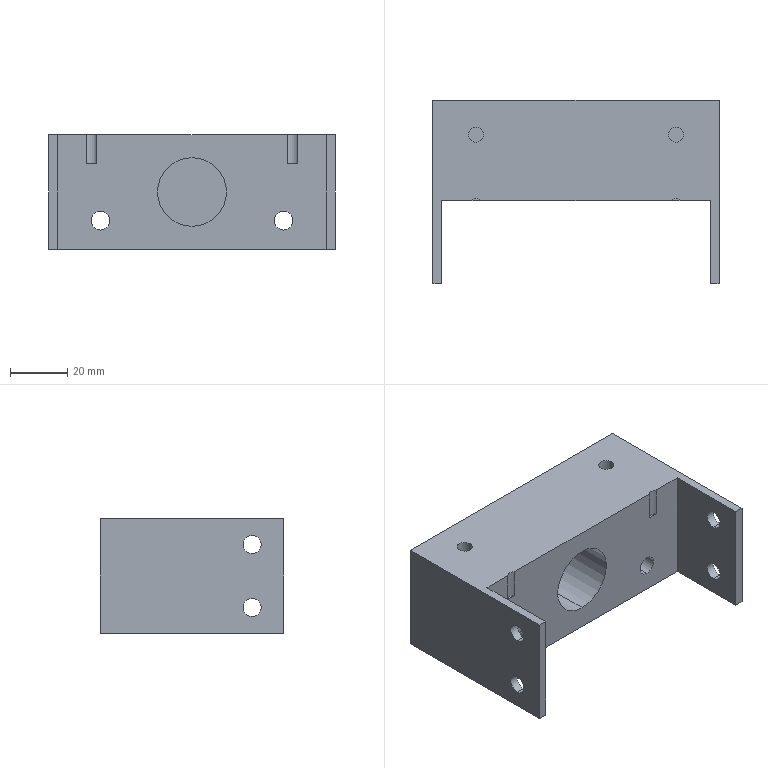Part | SolidWorks | features BaseBody 1 | 1 solid | 47 faces | box 100 x 64 x 40 mm | volume 128362 mm3 | cylinder 28 | plane 19 | commonest cylinder face diameters 4.3 x8 6.3 x8 5.3 x6 6.6 x4 24 x2
STEP:
#1=CARTESIAN_POINT('',(40.,24.8,9.85));
#2=VERTEX_POINT('',#1);
#3=CARTESIAN_POINT('',(40.,24.8,14.15));
#4=VERTEX_POINT('',#3);
#5=CARTESIAN_POINT('',(40.,24.8,12.));
#6=DIRECTION('',(0.,1.,0.));
#7=DIRECTION('',(0.,0.,1.));
#8=AXIS2_PLACEMENT_3D('',#5,#6,#7);
#9=CIRCLE('',#8,2.15);
#10=EDGE_CURVE('',#2,#4,#9,.T.);
#11=ORIENTED_EDGE('',*,*,#10,.F.);
#12=CARTESIAN_POINT('',(40.,32.,9.85));
#13=VERTEX_POINT('',#12);
#14=CARTESIAN_POINT('',(40.,24.8,9.85));
#15=DIRECTION('',(0.,1.,0.));
#16=VECTOR('',#15,1000.);
#17=LINE('',#14,#16);
#18=EDGE_CURVE('',#2,#13,#17,.T.);
#19=ORIENTED_EDGE('',*,*,#18,.T.);
#20=CARTESIAN_POINT('',(40.,32.,14.15));
#21=VERTEX_POINT('',#20);
#22=CARTESIAN_POINT('',(40.,32.,12.));
#23=DIRECTION('',(0.,-1.,0.));
#24=DIRECTION('',(0.,0.,1.));
#25=AXIS2_PLACEMENT_3D('',#22,#23,#24);
#26=CIRCLE('',#25,2.15);
#27=EDGE_CURVE('',#21,#13,#26,.T.);
#28=ORIENTED_EDGE('',*,*,#27,.F.);
#29=CARTESIAN_POINT('',(40.,24.8,14.15));
#30=DIRECTION('',(0.,1.,0.));
#31=VECTOR('',#30,1000.);
#32=LINE('',#29,#31);
#33=EDGE_CURVE('',#4,#21,#32,.T.);
#34=ORIENTED_EDGE('',*,*,#33,.F.);
#35=EDGE_LOOP('',(#11,#19,#28,#34));
#36=FACE_OUTER_BOUND('',#35,.T.);
#37=CARTESIAN_POINT('',(40.,24.8,12.));
#38=DIRECTION('',(0.,1.,0.));
#39=DIRECTION('',(0.,0.,1.));
#40=AXIS2_PLACEMENT_3D('',#37,#38,#39);
#41=CYLINDRICAL_SURFACE('',#40,2.15);
#42=ADVANCED_FACE('',(#36),#41,.F.);
#43=CARTESIAN_POINT('',(32.,-3.,-13.3));
#44=VERTEX_POINT('',#43);
#45=CARTESIAN_POINT('',(32.,-3.,-6.7));
#46=VERTEX_POINT('',#45);
#47=CARTESIAN_POINT('',(32.,-3.,-10.));
#48=DIRECTION('',(0.,1.,0.));
#49=DIRECTION('',(0.,0.,1.));
#50=AXIS2_PLACEMENT_3D('',#47,#48,#49);
#51=CIRCLE('',#50,3.3);
#52=EDGE_CURVE('',#44,#46,#51,.T.);
#53=ORIENTED_EDGE('',*,*,#52,.F.);
#54=CARTESIAN_POINT('',(32.,32.,-13.3));
#55=VERTEX_POINT('',#54);
#56=CARTESIAN_POINT('',(32.,-33.,-13.3));
#57=DIRECTION('',(0.,1.,0.));
#58=VECTOR('',#57,1000.);
#59=LINE('',#56,#58);
#60=EDGE_CURVE('',#44,#55,#59,.T.);
#61=ORIENTED_EDGE('',*,*,#60,.T.);
#62=CARTESIAN_POINT('',(32.,32.,-6.7));
#63=VERTEX_POINT('',#62);
#64=CARTESIAN_POINT('',(32.,32.,-10.));
#65=DIRECTION('',(0.,-1.,0.));
#66=DIRECTION('',(0.,0.,1.));
#67=AXIS2_PLACEMENT_3D('',#64,#65,#66);
#68=CIRCLE('',#67,3.3);
#69=EDGE_CURVE('',#63,#55,#68,.T.);
#70=ORIENTED_EDGE('',*,*,#69,.F.);
#71=CARTESIAN_POINT('',(32.,-33.,-6.7));
#72=DIRECTION('',(0.,1.,0.));
#73=VECTOR('',#72,1000.);
#74=LINE('',#71,#73);
#75=EDGE_CURVE('',#46,#63,#74,.T.);
#76=ORIENTED_EDGE('',*,*,#75,.F.);
#77=EDGE_LOOP('',(#53,#61,#70,#76));
#78=FACE_OUTER_BOUND('',#77,.T.);
#79=CARTESIAN_POINT('',(32.,-33.,-10.));
#80=DIRECTION('',(0.,1.,0.));
#81=DIRECTION('',(0.,0.,1.));
#82=AXIS2_PLACEMENT_3D('',#79,#80,#81);
#83=CYLINDRICAL_SURFACE('',#82,3.3);
#84=ADVANCED_FACE('',(#78),#83,.F.);
#85=CARTESIAN_POINT('',(40.,24.8,-14.15));
#86=VERTEX_POINT('',#85);
#87=CARTESIAN_POINT('',(40.,24.8,-9.85));
#88=VERTEX_POINT('',#87);
#89=CARTESIAN_POINT('',(40.,24.8,-12.));
#90=DIRECTION('',(0.,1.,0.));
#91=DIRECTION('',(0.,0.,1.));
#92=AXIS2_PLACEMENT_3D('',#89,#90,#91);
#93=CIRCLE('',#92,2.15);
#94=EDGE_CURVE('',#86,#88,#93,.T.);
#95=ORIENTED_EDGE('',*,*,#94,.F.);
#96=CARTESIAN_POINT('',(40.,32.,-14.15));
#97=VERTEX_POINT('',#96);
#98=CARTESIAN_POINT('',(40.,24.8,-14.15));
#99=DIRECTION('',(0.,1.,0.));
#100=VECTOR('',#99,1000.);
#101=LINE('',#98,#100);
#102=EDGE_CURVE('',#86,#97,#101,.T.);
#103=ORIENTED_EDGE('',*,*,#102,.T.);
#104=CARTESIAN_POINT('',(40.,32.,-9.85));
#105=VERTEX_POINT('',#104);
#106=CARTESIAN_POINT('',(40.,32.,-12.));
#107=DIRECTION('',(0.,-1.,0.));
#108=DIRECTION('',(0.,0.,1.));
#109=AXIS2_PLACEMENT_3D('',#106,#107,#108);
#110=CIRCLE('',#109,2.15);
#111=EDGE_CURVE('',#105,#97,#110,.T.);
#112=ORIENTED_EDGE('',*,*,#111,.F.);
#113=CARTESIAN_POINT('',(40.,24.8,-9.85));
#114=DIRECTION('',(0.,1.,0.));
#115=VECTOR('',#114,1000.);
#116=LINE('',#113,#115);
#117=EDGE_CURVE('',#88,#105,#116,.T.);
#118=ORIENTED_EDGE('',*,*,#117,.F.);
#119=EDGE_LOOP('',(#95,#103,#112,#118));
#120=FACE_OUTER_BOUND('',#119,.T.);
#121=CARTESIAN_POINT('',(40.,24.8,-12.));
#122=DIRECTION('',(0.,1.,0.));
#123=DIRECTION('',(0.,0.,1.));
#124=AXIS2_PLACEMENT_3D('',#121,#122,#123);
#125=CYLINDRICAL_SURFACE('',#124,2.15);
#126=ADVANCED_FACE('',(#120),#125,.F.);
#127=CARTESIAN_POINT('',(-40.,24.8,9.85));
#128=VERTEX_POINT('',#127);
#129=CARTESIAN_POINT('',(-40.,24.8,14.15));
#130=VERTEX_POINT('',#129);
#131=CARTESIAN_POINT('',(-40.,24.8,12.));
#132=DIRECTION('',(0.,1.,0.));
#133=DIRECTION('',(0.,0.,1.));
#134=AXIS2_PLACEMENT_3D('',#131,#132,#133);
#135=CIRCLE('',#134,2.15);
#136=EDGE_CURVE('',#128,#130,#135,.T.);
#137=ORIENTED_EDGE('',*,*,#136,.F.);
#138=CARTESIAN_POINT('',(-40.,32.,9.85));
#139=VERTEX_POINT('',#138);
#140=CARTESIAN_POINT('',(-40.,24.8,9.85));
#141=DIRECTION('',(0.,1.,0.));
#142=VECTOR('',#141,1000.);
#143=LINE('',#140,#142);
#144=EDGE_CURVE('',#128,#139,#143,.T.);
#145=ORIENTED_EDGE('',*,*,#144,.T.);
#146=CARTESIAN_POINT('',(-40.,32.,14.15));
#147=VERTEX_POINT('',#146);
#148=CARTESIAN_POINT('',(-40.,32.,12.));
#149=DIRECTION('',(0.,-1.,0.));
#150=DIRECTION('',(0.,0.,1.));
#151=AXIS2_PLACEMENT_3D('',#148,#149,#150);
#152=CIRCLE('',#151,2.15);
#153=EDGE_CURVE('',#147,#139,#152,.T.);
#154=ORIENTED_EDGE('',*,*,#153,.F.);
#155=CARTESIAN_POINT('',(-40.,24.8,14.15));
#156=DIRECTION('',(0.,1.,0.));
#157=VECTOR('',#156,1000.);
#158=LINE('',#155,#157);
#159=EDGE_CURVE('',#130,#147,#158,.T.);
#160=ORIENTED_EDGE('',*,*,#159,.F.);
#161=EDGE_LOOP('',(#137,#145,#154,#160));
#162=FACE_OUTER_BOUND('',#161,.T.);
#163=CARTESIAN_POINT('',(-40.,24.8,12.));
#164=DIRECTION('',(0.,1.,0.));
#165=DIRECTION('',(0.,0.,1.));
#166=AXIS2_PLACEMENT_3D('',#163,#164,#165);
#167=CYLINDRICAL_SURFACE('',#166,2.15);
#168=ADVANCED_FACE('',(#162),#167,.F.);
#169=CARTESIAN_POINT('',(-32.,-3.,-13.3));
#170=VERTEX_POINT('',#169);
#171=CARTESIAN_POINT('',(-32.,-3.,-6.7));
#172=VERTEX_POINT('',#171);
#173=CARTESIAN_POINT('',(-32.,-3.,-10.));
#174=DIRECTION('',(0.,1.,0.));
#175=DIRECTION('',(0.,0.,1.));
#176=AXIS2_PLACEMENT_3D('',#173,#174,#175);
#177=CIRCLE('',#176,3.3);
#178=EDGE_CURVE('',#170,#172,#177,.T.);
#179=ORIENTED_EDGE('',*,*,#178,.F.);
#180=CARTESIAN_POINT('',(-32.,32.,-13.3));
#181=VERTEX_POINT('',#180);
#182=CARTESIAN_POINT('',(-32.,-33.,-13.3));
#183=DIRECTION('',(0.,1.,0.));
#184=VECTOR('',#183,1000.);
#185=LINE('',#182,#184);
#186=EDGE_CURVE('',#170,#181,#185,.T.);
#187=ORIENTED_EDGE('',*,*,#186,.T.);
#188=CARTESIAN_POINT('',(-32.,32.,-6.7));
#189=VERTEX_POINT('',#188);
#190=CARTESIAN_POINT('',(-32.,32.,-10.));
#191=DIRECTION('',(0.,-1.,0.));
#192=DIRECTION('',(0.,0.,1.));
#193=AXIS2_PLACEMENT_3D('',#190,#191,#192);
#194=CIRCLE('',#193,3.3);
#195=EDGE_CURVE('',#189,#181,#194,.T.);
#196=ORIENTED_EDGE('',*,*,#195,.F.);
#197=CARTESIAN_POINT('',(-32.,-33.,-6.7));
#198=DIRECTION('',(0.,1.,0.));
#199=VECTOR('',#198,1000.);
#200=LINE('',#197,#199);
#201=EDGE_CURVE('',#172,#189,#200,.T.);
#202=ORIENTED_EDGE('',*,*,#201,.F.);
#203=EDGE_LOOP('',(#179,#187,#196,#202));
#204=FACE_OUTER_BOUND('',#203,.T.);
#205=CARTESIAN_POINT('',(-32.,-33.,-10.));
#206=DIRECTION('',(0.,1.,0.));
#207=DIRECTION('',(0.,0.,1.));
#208=AXIS2_PLACEMENT_3D('',#205,#206,#207);
#209=CYLINDRICAL_SURFACE('',#208,3.3);
#210=ADVANCED_FACE('',(#204),#209,.F.);
#211=CARTESIAN_POINT('',(-40.,24.8,-14.15));
#212=VERTEX_POINT('',#211);
#213=CARTESIAN_POINT('',(-40.,24.8,-9.85));
#214=VERTEX_POINT('',#213);
#215=CARTESIAN_POINT('',(-40.,24.8,-12.));
#216=DIRECTION('',(0.,1.,0.));
#217=DIRECTION('',(0.,0.,1.));
#218=AXIS2_PLACEMENT_3D('',#215,#216,#217);
#219=CIRCLE('',#218,2.15);
#220=EDGE_CURVE('',#212,#214,#219,.T.);
#221=ORIENTED_EDGE('',*,*,#220,.F.);
#222=CARTESIAN_POINT('',(-40.,32.,-14.15));
#223=VERTEX_POINT('',#222);
#224=CARTESIAN_POINT('',(-40.,24.8,-14.15));
#225=DIRECTION('',(0.,1.,0.));
#226=VECTOR('',#225,1000.);
#227=LINE('',#224,#226);
#228=EDGE_CURVE('',#212,#223,#227,.T.);
#229=ORIENTED_EDGE('',*,*,#228,.T.);
#230=CARTESIAN_POINT('',(-40.,32.,-9.85));
#231=VERTEX_POINT('',#230);
#232=CARTESIAN_POINT('',(-40.,32.,-12.));
#233=DIRECTION('',(0.,-1.,0.));
#234=DIRECTION('',(0.,0.,1.));
#235=AXIS2_PLACEMENT_3D('',#232,#233,#234);
#236=CIRCLE('',#235,2.15);
#237=EDGE_CURVE('',#231,#223,#236,.T.);
#238=ORIENTED_EDGE('',*,*,#237,.F.);
#239=CARTESIAN_POINT('',(-40.,24.8,-9.85));
#240=DIRECTION('',(0.,1.,0.));
#241=VECTOR('',#240,1000.);
#242=LINE('',#239,#241);
#243=EDGE_CURVE('',#214,#231,#242,.T.);
#244=ORIENTED_EDGE('',*,*,#243,.F.);
#245=EDGE_LOOP('',(#221,#229,#238,#244));
#246=FACE_OUTER_BOUND('',#245,.T.);
#247=CARTESIAN_POINT('',(-40.,24.8,-12.));
#248=DIRECTION('',(0.,1.,0.));
#249=DIRECTION('',(0.,0.,1.));
#250=AXIS2_PLACEMENT_3D('',#247,#248,#249);
#251=CYLINDRICAL_SURFACE('',#250,2.15);
#252=ADVANCED_FACE('',(#246),#251,.F.);
#253=CARTESIAN_POINT('',(47.,-21.,14.15));
#254=VERTEX_POINT('',#253);
#255=CARTESIAN_POINT('',(47.,-21.,7.85));
#256=VERTEX_POINT('',#255);
#257=CARTESIAN_POINT('',(47.,-21.,11.));
#258=DIRECTION('',(1.,0.,0.));
#259=DIRECTION('',(0.,0.,-1.));
#260=AXIS2_PLACEMENT_3D('',#257,#258,#259);
#261=CIRCLE('',#260,3.15);
#262=EDGE_CURVE('',#254,#256,#261,.T.);
#263=ORIENTED_EDGE('',*,*,#262,.F.);
#264=CARTESIAN_POINT('',(50.,-21.,14.15));
#265=VERTEX_POINT('',#264);
#266=CARTESIAN_POINT('',(-51.,-21.,14.15));
#267=DIRECTION('',(1.,0.,0.));
#268=VECTOR('',#267,1000.);
#269=LINE('',#266,#268);
#270=EDGE_CURVE('',#254,#265,#269,.T.);
#271=ORIENTED_EDGE('',*,*,#270,.T.);
#272=CARTESIAN_POINT('',(50.,-21.,7.85));
#273=VERTEX_POINT('',#272);
#274=CARTESIAN_POINT('',(50.,-21.,11.));
#275=DIRECTION('',(-1.,0.,0.));
#276=DIRECTION('',(0.,0.,-1.));
#277=AXIS2_PLACEMENT_3D('',#274,#275,#276);
#278=CIRCLE('',#277,3.15);
#279=EDGE_CURVE('',#273,#265,#278,.T.);
#280=ORIENTED_EDGE('',*,*,#279,.F.);
#281=CARTESIAN_POINT('',(-51.,-21.,7.85));
#282=DIRECTION('',(1.,0.,0.));
#283=VECTOR('',#282,1000.);
#284=LINE('',#281,#283);
#285=EDGE_CURVE('',#256,#273,#284,.T.);
#286=ORIENTED_EDGE('',*,*,#285,.F.);
#287=EDGE_LOOP('',(#263,#271,#280,#286));
#288=FACE_OUTER_BOUND('',#287,.T.);
#289=CARTESIAN_POINT('',(-51.,-21.,11.));
#290=DIRECTION('',(1.,0.,0.));
#291=DIRECTION('',(0.,0.,-1.));
#292=AXIS2_PLACEMENT_3D('',#289,#290,#291);
#293=CYLINDRICAL_SURFACE('',#292,3.15);
#294=ADVANCED_FACE('',(#288),#293,.F.);
#295=CARTESIAN_POINT('',(47.,-21.,-7.85));
#296=VERTEX_POINT('',#295);
#297=CARTESIAN_POINT('',(47.,-21.,-14.15));
#298=VERTEX_POINT('',#297);
#299=CARTESIAN_POINT('',(47.,-21.,-11.));
#300=DIRECTION('',(1.,0.,0.));
#301=DIRECTION('',(0.,0.,-1.));
#302=AXIS2_PLACEMENT_3D('',#299,#300,#301);
#303=CIRCLE('',#302,3.15);
#304=EDGE_CURVE('',#296,#298,#303,.T.);
#305=ORIENTED_EDGE('',*,*,#304,.F.);
#306=CARTESIAN_POINT('',(50.,-21.,-7.85));
#307=VERTEX_POINT('',#306);
#308=CARTESIAN_POINT('',(-51.,-21.,-7.85));
#309=DIRECTION('',(1.,0.,0.));
#310=VECTOR('',#309,1000.);
#311=LINE('',#308,#310);
#312=EDGE_CURVE('',#296,#307,#311,.T.);
#313=ORIENTED_EDGE('',*,*,#312,.T.);
#314=CARTESIAN_POINT('',(50.,-21.,-14.15));
#315=VERTEX_POINT('',#314);
#316=CARTESIAN_POINT('',(50.,-21.,-11.));
#317=DIRECTION('',(-1.,0.,0.));
#318=DIRECTION('',(0.,0.,-1.));
#319=AXIS2_PLACEMENT_3D('',#316,#317,#318);
#320=CIRCLE('',#319,3.15);
#321=EDGE_CURVE('',#315,#307,#320,.T.);
#322=ORIENTED_EDGE('',*,*,#321,.F.);
#323=CARTESIAN_POINT('',(-51.,-21.,-14.15));
#324=DIRECTION('',(1.,0.,0.));
#325=VECTOR('',#324,1000.);
#326=LINE('',#323,#325);
#327=EDGE_CURVE('',#298,#315,#326,.T.);
#328=ORIENTED_EDGE('',*,*,#327,.F.);
#329=EDGE_LOOP('',(#305,#313,#322,#328));
#330=FACE_OUTER_BOUND('',#329,.T.);
#331=CARTESIAN_POINT('',(-51.,-21.,-11.));
#332=DIRECTION('',(1.,0.,0.));
#333=DIRECTION('',(0.,0.,-1.));
#334=AXIS2_PLACEMENT_3D('',#331,#332,#333);
#335=CYLINDRICAL_SURFACE('',#334,3.15);
#336=ADVANCED_FACE('',(#330),#335,.F.);
#337=CARTESIAN_POINT('',(32.35,20.,9.8));
#338=VERTEX_POINT('',#337);
#339=CARTESIAN_POINT('',(37.65,20.,9.8));
#340=VERTEX_POINT('',#339);
#341=CARTESIAN_POINT('',(35.,20.,9.8));
#342=DIRECTION('',(0.,0.,1.));
#343=DIRECTION('',(1.,0.,0.));
#344=AXIS2_PLACEMENT_3D('',#341,#342,#343);
#345=CIRCLE('',#344,2.65);
#346=EDGE_CURVE('',#338,#340,#345,.T.);
#347=ORIENTED_EDGE('',*,*,#346,.F.);
#348=CARTESIAN_POINT('',(32.35,20.,20.));
#349=VERTEX_POINT('',#348);
#350=CARTESIAN_POINT('',(32.35,20.,9.8));
#351=DIRECTION('',(0.,0.,1.));
#352=VECTOR('',#351,1000.);
#353=LINE('',#350,#352);
#354=EDGE_CURVE('',#338,#349,#353,.T.);
#355=ORIENTED_EDGE('',*,*,#354,.T.);
#356=CARTESIAN_POINT('',(37.65,20.,20.));
#357=VERTEX_POINT('',#356);
#358=CARTESIAN_POINT('',(35.,20.,20.));
#359=DIRECTION('',(0.,0.,-1.));
#360=DIRECTION('',(1.,0.,0.));
#361=AXIS2_PLACEMENT_3D('',#358,#359,#360);
#362=CIRCLE('',#361,2.65);
#363=EDGE_CURVE('',#357,#349,#362,.T.);
#364=ORIENTED_EDGE('',*,*,#363,.F.);
#365=CARTESIAN_POINT('',(37.65,20.,9.8));
#366=DIRECTION('',(0.,0.,1.));
#367=VECTOR('',#366,1000.);
#368=LINE('',#365,#367);
#369=EDGE_CURVE('',#340,#357,#368,.T.);
#370=ORIENTED_EDGE('',*,*,#369,.F.);
#371=EDGE_LOOP('',(#347,#355,#364,#370));
#372=FACE_OUTER_BOUND('',#371,.T.);
#373=CARTESIAN_POINT('',(35.,20.,9.8));
#374=DIRECTION('',(0.,0.,1.));
#375=DIRECTION('',(1.,0.,0.));
#376=AXIS2_PLACEMENT_3D('',#373,#374,#375);
#377=CYLINDRICAL_SURFACE('',#376,2.65);
#378=ADVANCED_FACE('',(#372),#377,.F.);
#379=CARTESIAN_POINT('',(-37.65,20.,9.8));
#380=VERTEX_POINT('',#379);
#381=CARTESIAN_POINT('',(-32.35,20.,9.8));
#382=VERTEX_POINT('',#381);
#383=CARTESIAN_POINT('',(-35.,20.,9.8));
#384=DIRECTION('',(0.,0.,1.));
#385=DIRECTION('',(1.,0.,0.));
#386=AXIS2_PLACEMENT_3D('',#383,#384,#385);
#387=CIRCLE('',#386,2.65);
#388=EDGE_CURVE('',#380,#382,#387,.T.);
#389=ORIENTED_EDGE('',*,*,#388,.F.);
#390=CARTESIAN_POINT('',(-37.65,20.,20.));
#391=VERTEX_POINT('',#390);
#392=CARTESIAN_POINT('',(-37.65,20.,9.8));
#393=DIRECTION('',(0.,0.,1.));
#394=VECTOR('',#393,1000.);
#395=LINE('',#392,#394);
#396=EDGE_CURVE('',#380,#391,#395,.T.);
#397=ORIENTED_EDGE('',*,*,#396,.T.);
#398=CARTESIAN_POINT('',(-32.35,20.,20.));
#399=VERTEX_POINT('',#398);
#400=CARTESIAN_POINT('',(-35.,20.,20.));
#401=DIRECTION('',(0.,0.,-1.));
#402=DIRECTION('',(1.,0.,0.));
#403=AXIS2_PLACEMENT_3D('',#400,#401,#402);
#404=CIRCLE('',#403,2.65);
#405=EDGE_CURVE('',#399,#391,#404,.T.);
#406=ORIENTED_EDGE('',*,*,#405,.F.);
#407=CARTESIAN_POINT('',(-32.35,20.,9.8));
#408=DIRECTION('',(0.,0.,1.));
#409=VECTOR('',#408,1000.);
#410=LINE('',#407,#409);
#411=EDGE_CURVE('',#382,#399,#410,.T.);
#412=ORIENTED_EDGE('',*,*,#411,.F.);
#413=EDGE_LOOP('',(#389,#397,#406,#412));
#414=FACE_OUTER_BOUND('',#413,.T.);
#415=CARTESIAN_POINT('',(-35.,20.,9.8));
#416=DIRECTION('',(0.,0.,1.));
#417=DIRECTION('',(1.,0.,0.));
#418=AXIS2_PLACEMENT_3D('',#415,#416,#417);
#419=CYLINDRICAL_SURFACE('',#418,2.65);
#420=ADVANCED_FACE('',(#414),#419,.F.);
#421=CARTESIAN_POINT('',(-50.,-21.,7.85));
#422=VERTEX_POINT('',#421);
#423=CARTESIAN_POINT('',(-50.,-21.,14.15));
#424=VERTEX_POINT('',#423);
#425=CARTESIAN_POINT('',(-50.,-21.,11.));
#426=DIRECTION('',(-1.,0.,0.));
#427=DIRECTION('',(0.,0.,-1.));
#428=AXIS2_PLACEMENT_3D('',#425,#426,#427);
#429=CIRCLE('',#428,3.15);
#430=EDGE_CURVE('',#422,#424,#429,.T.);
#431=ORIENTED_EDGE('',*,*,#430,.T.);
#432=CARTESIAN_POINT('',(-47.,-21.,14.15));
#433=VERTEX_POINT('',#432);
#434=CARTESIAN_POINT('',(-51.,-21.,14.15));
#435=DIRECTION('',(1.,0.,0.));
#436=VECTOR('',#435,1000.);
#437=LINE('',#434,#436);
#438=EDGE_CURVE('',#424,#433,#437,.T.);
#439=ORIENTED_EDGE('',*,*,#438,.T.);
#440=CARTESIAN_POINT('',(-47.,-21.,7.85));
#441=VERTEX_POINT('',#440);
#442=CARTESIAN_POINT('',(-47.,-21.,11.));
#443=DIRECTION('',(-1.,0.,0.));
#444=DIRECTION('',(0.,0.,-1.));
#445=AXIS2_PLACEMENT_3D('',#442,#443,#444);
#446=CIRCLE('',#445,3.15);
#447=EDGE_CURVE('',#441,#433,#446,.T.);
#448=ORIENTED_EDGE('',*,*,#447,.F.);
#449=CARTESIAN_POINT('',(-51.,-21.,7.85));
#450=DIRECTION('',(1.,0.,0.));
#451=VECTOR('',#450,1000.);
#452=LINE('',#449,#451);
#453=EDGE_CURVE('',#422,#441,#452,.T.);
#454=ORIENTED_EDGE('',*,*,#453,.F.);
#455=EDGE_LOOP('',(#431,#439,#448,#454));
#456=FACE_OUTER_BOUND('',#455,.T.);
#457=CARTESIAN_POINT('',(-51.,-21.,11.));
#458=DIRECTION('',(1.,0.,0.));
#459=DIRECTION('',(0.,0.,-1.));
#460=AXIS2_PLACEMENT_3D('',#457,#458,#459);
#461=CYLINDRICAL_SURFACE('',#460,3.15);
#462=ADVANCED_FACE('',(#456),#461,.F.);
#463=CARTESIAN_POINT('',(-50.,-21.,-14.15));
#464=VERTEX_POINT('',#463);
#465=CARTESIAN_POINT('',(-50.,-21.,-7.85));
#466=VERTEX_POINT('',#465);
#467=CARTESIAN_POINT('',(-50.,-21.,-11.));
#468=DIRECTION('',(-1.,0.,0.));
#469=DIRECTION('',(0.,0.,-1.));
#470=AXIS2_PLACEMENT_3D('',#467,#468,#469);
#471=CIRCLE('',#470,3.15);
#472=EDGE_CURVE('',#464,#466,#471,.T.);
#473=ORIENTED_EDGE('',*,*,#472,.T.);
#474=CARTESIAN_POINT('',(-47.,-21.,-7.85));
#475=VERTEX_POINT('',#474);
#476=CARTESIAN_POINT('',(-51.,-21.,-7.85));
#477=DIRECTION('',(1.,0.,0.));
#478=VECTOR('',#477,1000.);
#479=LINE('',#476,#478);
#480=EDGE_CURVE('',#466,#475,#479,.T.);
#481=ORIENTED_EDGE('',*,*,#480,.T.);
#482=CARTESIAN_POINT('',(-47.,-21.,-14.15));
#483=VERTEX_POINT('',#482);
#484=CARTESIAN_POINT('',(-47.,-21.,-11.));
#485=DIRECTION('',(-1.,0.,0.));
#486=DIRECTION('',(0.,0.,-1.));
#487=AXIS2_PLACEMENT_3D('',#484,#485,#486);
#488=CIRCLE('',#487,3.15);
#489=EDGE_CURVE('',#483,#475,#488,.T.);
#490=ORIENTED_EDGE('',*,*,#489,.F.);
#491=CARTESIAN_POINT('',(-51.,-21.,-14.15));
#492=DIRECTION('',(1.,0.,0.));
#493=VECTOR('',#492,1000.);
#494=LINE('',#491,#493);
#495=EDGE_CURVE('',#464,#483,#494,.T.);
#496=ORIENTED_EDGE('',*,*,#495,.F.);
#497=EDGE_LOOP('',(#473,#481,#490,#496));
#498=FACE_OUTER_BOUND('',#497,.T.);
#499=CARTESIAN_POINT('',(-51.,-21.,-11.));
#500=DIRECTION('',(1.,0.,0.));
#501=DIRECTION('',(0.,0.,-1.));
#502=AXIS2_PLACEMENT_3D('',#499,#500,#501);
#503=CYLINDRICAL_SURFACE('',#502,3.15);
#504=ADVANCED_FACE('',(#498),#503,.F.);
#505=CARTESIAN_POINT('',(0.,-3.,12.));
#506=VERTEX_POINT('',#505);
#507=CARTESIAN_POINT('',(0.,-3.,-12.));
#508=VERTEX_POINT('',#507);
#509=CARTESIAN_POINT('',(0.,-3.,0.));
#510=DIRECTION('',(0.,-1.,0.));
#511=DIRECTION('',(0.,0.,1.));
#512=AXIS2_PLACEMENT_3D('',#509,#510,#511);
#513=CIRCLE('',#512,12.);
#514=EDGE_CURVE('',#506,#508,#513,.T.);
#515=ORIENTED_EDGE('',*,*,#514,.T.);
#516=CARTESIAN_POINT('',(0.,30.,-12.));
#517=VERTEX_POINT('',#516);
#518=CARTESIAN_POINT('',(0.,-14.,-12.));
#519=DIRECTION('',(0.,1.,0.));
#520=VECTOR('',#519,1000.);
#521=LINE('',#518,#520);
#522=EDGE_CURVE('',#508,#517,#521,.T.);
#523=ORIENTED_EDGE('',*,*,#522,.T.);
#524=CARTESIAN_POINT('',(0.,30.,12.));
#525=VERTEX_POINT('',#524);
#526=CARTESIAN_POINT('',(0.,30.,0.));
#527=DIRECTION('',(0.,-1.,0.));
#528=DIRECTION('',(0.,0.,1.));
#529=AXIS2_PLACEMENT_3D('',#526,#527,#528);
#530=CIRCLE('',#529,12.);
#531=EDGE_CURVE('',#525,#517,#530,.T.);
#532=ORIENTED_EDGE('',*,*,#531,.F.);
#533=CARTESIAN_POINT('',(0.,-14.,12.));
#534=DIRECTION('',(0.,1.,0.));
#535=VECTOR('',#534,1000.);
#536=LINE('',#533,#535);
#537=EDGE_CURVE('',#506,#525,#536,.T.);
#538=ORIENTED_EDGE('',*,*,#537,.F.);
#539=EDGE_LOOP('',(#515,#523,#532,#538));
#540=FACE_OUTER_BOUND('',#539,.T.);
#541=CARTESIAN_POINT('',(0.,-14.,0.));
#542=DIRECTION('',(0.,1.,0.));
#543=DIRECTION('',(0.,0.,1.));
#544=AXIS2_PLACEMENT_3D('',#541,#542,#543);
#545=CYLINDRICAL_SURFACE('',#544,12.);
#546=ADVANCED_FACE('',(#540),#545,.F.);
#547=ORIENTED_EDGE('',*,*,#27,.T.);
#548=CARTESIAN_POINT('',(40.,32.,12.));
#549=DIRECTION('',(0.,-1.,0.));
#550=DIRECTION('',(0.,0.,1.));
#551=AXIS2_PLACEMENT_3D('',#548,#549,#550);
#552=CIRCLE('',#551,2.15);
#553=EDGE_CURVE('',#13,#21,#552,.T.);
#554=ORIENTED_EDGE('',*,*,#553,.T.);
#555=EDGE_LOOP('',(#547,#554));
#556=FACE_BOUND('',#555,.T.);
#557=ORIENTED_EDGE('',*,*,#69,.T.);
#558=CARTESIAN_POINT('',(32.,32.,-10.));
#559=DIRECTION('',(0.,-1.,0.));
#560=DIRECTION('',(0.,0.,1.));
#561=AXIS2_PLACEMENT_3D('',#558,#559,#560);
#562=CIRCLE('',#561,3.3);
#563=EDGE_CURVE('',#55,#63,#562,.T.);
#564=ORIENTED_EDGE('',*,*,#563,.T.);
#565=EDGE_LOOP('',(#557,#564));
#566=FACE_BOUND('',#565,.T.);
#567=ORIENTED_EDGE('',*,*,#111,.T.);
#568=CARTESIAN_POINT('',(40.,32.,-12.));
#569=DIRECTION('',(0.,-1.,0.));
#570=DIRECTION('',(0.,0.,1.));
#571=AXIS2_PLACEMENT_3D('',#568,#569,#570);
#572=CIRCLE('',#571,2.15);
#573=EDGE_CURVE('',#97,#105,#572,.T.);
#574=ORIENTED_EDGE('',*,*,#573,.T.);
#575=EDGE_LOOP('',(#567,#574));
#576=FACE_BOUND('',#575,.T.);
#577=ORIENTED_EDGE('',*,*,#153,.T.);
#578=CARTESIAN_POINT('',(-40.,32.,12.));
#579=DIRECTION('',(0.,-1.,0.));
#580=DIRECTION('',(0.,0.,1.));
#581=AXIS2_PLACEMENT_3D('',#578,#579,#580);
#582=CIRCLE('',#581,2.15);
#583=EDGE_CURVE('',#139,#147,#582,.T.);
#584=ORIENTED_EDGE('',*,*,#583,.T.);
#585=EDGE_LOOP('',(#577,#584));
#586=FACE_BOUND('',#585,.T.);
#587=ORIENTED_EDGE('',*,*,#195,.T.);
#588=CARTESIAN_POINT('',(-32.,32.,-10.));
#589=DIRECTION('',(0.,-1.,0.));
#590=DIRECTION('',(0.,0.,1.));
#591=AXIS2_PLACEMENT_3D('',#588,#589,#590);
#592=CIRCLE('',#591,3.3);
#593=EDGE_CURVE('',#181,#189,#592,.T.);
#594=ORIENTED_EDGE('',*,*,#593,.T.);
#595=EDGE_LOOP('',(#587,#594));
#596=FACE_BOUND('',#595,.T.);
#597=ORIENTED_EDGE('',*,*,#237,.T.);
#598=CARTESIAN_POINT('',(-40.,32.,-12.));
#599=DIRECTION('',(0.,-1.,0.));
#600=DIRECTION('',(0.,0.,1.));
#601=AXIS2_PLACEMENT_3D('',#598,#599,#600);
#602=CIRCLE('',#601,2.15);
#603=EDGE_CURVE('',#223,#231,#602,.T.);
#604=ORIENTED_EDGE('',*,*,#603,.T.);
#605=EDGE_LOOP('',(#597,#604));
#606=FACE_BOUND('',#605,.T.);
#607=CARTESIAN_POINT('',(-50.,32.,20.));
#608=VERTEX_POINT('',#607);
#609=CARTESIAN_POINT('',(50.,32.,20.));
#610=VERTEX_POINT('',#609);
#611=CARTESIAN_POINT('',(-50.,32.,20.));
#612=DIRECTION('',(1.,0.,0.));
#613=VECTOR('',#612,1000.);
#614=LINE('',#611,#613);
#615=EDGE_CURVE('',#608,#610,#614,.T.);
#616=ORIENTED_EDGE('',*,*,#615,.T.);
#617=CARTESIAN_POINT('',(50.,32.,-20.));
#618=VERTEX_POINT('',#617);
#619=CARTESIAN_POINT('',(50.,32.,-20.));
#620=DIRECTION('',(0.,0.,-1.));
#621=VECTOR('',#620,1000.);
#622=LINE('',#619,#621);
#623=EDGE_CURVE('',#610,#618,#622,.T.);
#624=ORIENTED_EDGE('',*,*,#623,.T.);
#625=CARTESIAN_POINT('',(-50.,32.,-20.));
#626=VERTEX_POINT('',#625);
#627=CARTESIAN_POINT('',(-50.,32.,-20.));
#628=DIRECTION('',(-1.,0.,0.));
#629=VECTOR('',#628,1000.);
#630=LINE('',#627,#629);
#631=EDGE_CURVE('',#618,#626,#630,.T.);
#632=ORIENTED_EDGE('',*,*,#631,.T.);
#633=CARTESIAN_POINT('',(-50.,32.,-20.));
#634=DIRECTION('',(0.,0.,1.));
#635=VECTOR('',#634,1000.);
#636=LINE('',#633,#635);
#637=EDGE_CURVE('',#626,#608,#636,.T.);
#638=ORIENTED_EDGE('',*,*,#637,.T.);
#639=EDGE_LOOP('',(#616,#624,#632,#638));
#640=FACE_OUTER_BOUND('',#639,.T.);
#641=CARTESIAN_POINT('',(-50.,32.,-20.));
#642=DIRECTION('',(0.,1.,0.));
#643=DIRECTION('',(0.,0.,1.));
#644=AXIS2_PLACEMENT_3D('',#641,#642,#643);
#645=PLANE('',#644);
#646=ADVANCED_FACE('',(#556,#566,#576,#586,#596,#606,#640),#645,.T.);
#647=ORIENTED_EDGE('',*,*,#18,.F.);
#648=CARTESIAN_POINT('',(40.,24.8,12.));
#649=DIRECTION('',(0.,1.,0.));
#650=DIRECTION('',(0.,0.,1.));
#651=AXIS2_PLACEMENT_3D('',#648,#649,#650);
#652=CIRCLE('',#651,2.15);
#653=EDGE_CURVE('',#4,#2,#652,.T.);
#654=ORIENTED_EDGE('',*,*,#653,.F.);
#655=ORIENTED_EDGE('',*,*,#33,.T.);
#656=ORIENTED_EDGE('',*,*,#553,.F.);
#657=EDGE_LOOP('',(#647,#654,#655,#656));
#658=FACE_OUTER_BOUND('',#657,.T.);
#659=CARTESIAN_POINT('',(40.,24.8,12.));
#660=DIRECTION('',(0.,1.,0.));
#661=DIRECTION('',(0.,0.,1.));
#662=AXIS2_PLACEMENT_3D('',#659,#660,#661);
#663=CYLINDRICAL_SURFACE('',#662,2.15);
#664=ADVANCED_FACE('',(#658),#663,.F.);
#665=ORIENTED_EDGE('',*,*,#60,.F.);
#666=CARTESIAN_POINT('',(32.,-3.,-10.));
#667=DIRECTION('',(0.,1.,0.));
#668=DIRECTION('',(0.,0.,1.));
#669=AXIS2_PLACEMENT_3D('',#666,#667,#668);
#670=CIRCLE('',#669,3.3);
#671=EDGE_CURVE('',#46,#44,#670,.T.);
#672=ORIENTED_EDGE('',*,*,#671,.F.);
#673=ORIENTED_EDGE('',*,*,#75,.T.);
#674=ORIENTED_EDGE('',*,*,#563,.F.);
#675=EDGE_LOOP('',(#665,#672,#673,#674));
#676=FACE_OUTER_BOUND('',#675,.T.);
#677=CARTESIAN_POINT('',(32.,-33.,-10.));
#678=DIRECTION('',(0.,1.,0.));
#679=DIRECTION('',(0.,0.,1.));
#680=AXIS2_PLACEMENT_3D('',#677,#678,#679);
#681=CYLINDRICAL_SURFACE('',#680,3.3);
#682=ADVANCED_FACE('',(#676),#681,.F.);
#683=ORIENTED_EDGE('',*,*,#102,.F.);
#684=CARTESIAN_POINT('',(40.,24.8,-12.));
#685=DIRECTION('',(0.,1.,0.));
#686=DIRECTION('',(0.,0.,1.));
#687=AXIS2_PLACEMENT_3D('',#684,#685,#686);
#688=CIRCLE('',#687,2.15);
#689=EDGE_CURVE('',#88,#86,#688,.T.);
#690=ORIENTED_EDGE('',*,*,#689,.F.);
#691=ORIENTED_EDGE('',*,*,#117,.T.);
#692=ORIENTED_EDGE('',*,*,#573,.F.);
#693=EDGE_LOOP('',(#683,#690,#691,#692));
#694=FACE_OUTER_BOUND('',#693,.T.);
#695=CARTESIAN_POINT('',(40.,24.8,-12.));
#696=DIRECTION('',(0.,1.,0.));
#697=DIRECTION('',(0.,0.,1.));
#698=AXIS2_PLACEMENT_3D('',#695,#696,#697);
#699=CYLINDRICAL_SURFACE('',#698,2.15);
#700=ADVANCED_FACE('',(#694),#699,.F.);
#701=ORIENTED_EDGE('',*,*,#144,.F.);
#702=CARTESIAN_POINT('',(-40.,24.8,12.));
#703=DIRECTION('',(0.,1.,0.));
#704=DIRECTION('',(0.,0.,1.));
#705=AXIS2_PLACEMENT_3D('',#702,#703,#704);
#706=CIRCLE('',#705,2.15);
#707=EDGE_CURVE('',#130,#128,#706,.T.);
#708=ORIENTED_EDGE('',*,*,#707,.F.);
#709=ORIENTED_EDGE('',*,*,#159,.T.);
#710=ORIENTED_EDGE('',*,*,#583,.F.);
#711=EDGE_LOOP('',(#701,#708,#709,#710));
#712=FACE_OUTER_BOUND('',#711,.T.);
#713=CARTESIAN_POINT('',(-40.,24.8,12.));
#714=DIRECTION('',(0.,1.,0.));
#715=DIRECTION('',(0.,0.,1.));
#716=AXIS2_PLACEMENT_3D('',#713,#714,#715);
#717=CYLINDRICAL_SURFACE('',#716,2.15);
#718=ADVANCED_FACE('',(#712),#717,.F.);
#719=ORIENTED_EDGE('',*,*,#186,.F.);
#720=CARTESIAN_POINT('',(-32.,-3.,-10.));
#721=DIRECTION('',(0.,1.,0.));
#722=DIRECTION('',(0.,0.,1.));
#723=AXIS2_PLACEMENT_3D('',#720,#721,#722);
#724=CIRCLE('',#723,3.3);
#725=EDGE_CURVE('',#172,#170,#724,.T.);
#726=ORIENTED_EDGE('',*,*,#725,.F.);
#727=ORIENTED_EDGE('',*,*,#201,.T.);
#728=ORIENTED_EDGE('',*,*,#593,.F.);
#729=EDGE_LOOP('',(#719,#726,#727,#728));
#730=FACE_OUTER_BOUND('',#729,.T.);
#731=CARTESIAN_POINT('',(-32.,-33.,-10.));
#732=DIRECTION('',(0.,1.,0.));
#733=DIRECTION('',(0.,0.,1.));
#734=AXIS2_PLACEMENT_3D('',#731,#732,#733);
#735=CYLINDRICAL_SURFACE('',#734,3.3);
#736=ADVANCED_FACE('',(#730),#735,.F.);
#737=ORIENTED_EDGE('',*,*,#228,.F.);
#738=CARTESIAN_POINT('',(-40.,24.8,-12.));
#739=DIRECTION('',(0.,1.,0.));
#740=DIRECTION('',(0.,0.,1.));
#741=AXIS2_PLACEMENT_3D('',#738,#739,#740);
#742=CIRCLE('',#741,2.15);
#743=EDGE_CURVE('',#214,#212,#742,.T.);
#744=ORIENTED_EDGE('',*,*,#743,.F.);
#745=ORIENTED_EDGE('',*,*,#243,.T.);
#746=ORIENTED_EDGE('',*,*,#603,.F.);
#747=EDGE_LOOP('',(#737,#744,#745,#746));
#748=FACE_OUTER_BOUND('',#747,.T.);
#749=CARTESIAN_POINT('',(-40.,24.8,-12.));
#750=DIRECTION('',(0.,1.,0.));
#751=DIRECTION('',(0.,0.,1.));
#752=AXIS2_PLACEMENT_3D('',#749,#750,#751);
#753=CYLINDRICAL_SURFACE('',#752,2.15);
#754=ADVANCED_FACE('',(#748),#753,.F.);
#755=ORIENTED_EDGE('',*,*,#279,.T.);
#756=CARTESIAN_POINT('',(50.,-21.,11.));
#757=DIRECTION('',(-1.,0.,0.));
#758=DIRECTION('',(0.,0.,-1.));
#759=AXIS2_PLACEMENT_3D('',#756,#757,#758);
#760=CIRCLE('',#759,3.15);
#761=EDGE_CURVE('',#265,#273,#760,.T.);
#762=ORIENTED_EDGE('',*,*,#761,.T.);
#763=EDGE_LOOP('',(#755,#762));
#764=FACE_BOUND('',#763,.T.);
#765=ORIENTED_EDGE('',*,*,#321,.T.);
#766=CARTESIAN_POINT('',(50.,-21.,-11.));
#767=DIRECTION('',(-1.,0.,0.));
#768=DIRECTION('',(0.,0.,-1.));
#769=AXIS2_PLACEMENT_3D('',#766,#767,#768);
#770=CIRCLE('',#769,3.15);
#771=EDGE_CURVE('',#307,#315,#770,.T.);
#772=ORIENTED_EDGE('',*,*,#771,.T.);
#773=EDGE_LOOP('',(#765,#772));
#774=FACE_BOUND('',#773,.T.);
#775=ORIENTED_EDGE('',*,*,#623,.F.);
#776=CARTESIAN_POINT('',(50.,-32.,20.));
#777=VERTEX_POINT('',#776);
#778=CARTESIAN_POINT('',(50.,-32.,20.));
#779=DIRECTION('',(0.,-1.,0.));
#780=VECTOR('',#779,1000.);
#781=LINE('',#778,#780);
#782=EDGE_CURVE('',#610,#777,#781,.T.);
#783=ORIENTED_EDGE('',*,*,#782,.T.);
#784=CARTESIAN_POINT('',(50.,-32.,-20.));
#785=VERTEX_POINT('',#784);
#786=CARTESIAN_POINT('',(50.,-32.,-20.));
#787=DIRECTION('',(0.,0.,-1.));
#788=VECTOR('',#787,1000.);
#789=LINE('',#786,#788);
#790=EDGE_CURVE('',#777,#785,#789,.T.);
#791=ORIENTED_EDGE('',*,*,#790,.T.);
#792=CARTESIAN_POINT('',(50.,-32.,-20.));
#793=DIRECTION('',(0.,1.,0.));
#794=VECTOR('',#793,1000.);
#795=LINE('',#792,#794);
#796=EDGE_CURVE('',#785,#618,#795,.T.);
#797=ORIENTED_EDGE('',*,*,#796,.T.);
#798=EDGE_LOOP('',(#775,#783,#791,#797));
#799=FACE_OUTER_BOUND('',#798,.T.);
#800=CARTESIAN_POINT('',(50.,-32.,-20.));
#801=DIRECTION('',(1.,0.,0.));
#802=DIRECTION('',(0.,0.,-1.));
#803=AXIS2_PLACEMENT_3D('',#800,#801,#802);
#804=PLANE('',#803);
#805=ADVANCED_FACE('',(#764,#774,#799),#804,.T.);
#806=ORIENTED_EDGE('',*,*,#363,.T.);
#807=CARTESIAN_POINT('',(35.,20.,20.));
#808=DIRECTION('',(0.,0.,-1.));
#809=DIRECTION('',(1.,0.,0.));
#810=AXIS2_PLACEMENT_3D('',#807,#808,#809);
#811=CIRCLE('',#810,2.65);
#812=EDGE_CURVE('',#349,#357,#811,.T.);
#813=ORIENTED_EDGE('',*,*,#812,.T.);
#814=EDGE_LOOP('',(#806,#813));
#815=FACE_BOUND('',#814,.T.);
#816=ORIENTED_EDGE('',*,*,#405,.T.);
#817=CARTESIAN_POINT('',(-35.,20.,20.));
#818=DIRECTION('',(0.,0.,-1.));
#819=DIRECTION('',(1.,0.,0.));
#820=AXIS2_PLACEMENT_3D('',#817,#818,#819);
#821=CIRCLE('',#820,2.65);
#822=EDGE_CURVE('',#391,#399,#821,.T.);
#823=ORIENTED_EDGE('',*,*,#822,.T.);
#824=EDGE_LOOP('',(#816,#823));
#825=FACE_BOUND('',#824,.T.);
#826=CARTESIAN_POINT('',(47.,-32.,20.));
#827=VERTEX_POINT('',#826);
#828=CARTESIAN_POINT('',(-50.,-32.,20.));
#829=DIRECTION('',(1.,0.,0.));
#830=VECTOR('',#829,1000.);
#831=LINE('',#828,#830);
#832=EDGE_CURVE('',#827,#777,#831,.T.);
#833=ORIENTED_EDGE('',*,*,#832,.T.);
#834=ORIENTED_EDGE('',*,*,#782,.F.);
#835=ORIENTED_EDGE('',*,*,#615,.F.);
#836=CARTESIAN_POINT('',(-50.,-32.,20.));
#837=VERTEX_POINT('',#836);
#838=CARTESIAN_POINT('',(-50.,-32.,20.));
#839=DIRECTION('',(0.,-1.,0.));
#840=VECTOR('',#839,1000.);
#841=LINE('',#838,#840);
#842=EDGE_CURVE('',#608,#837,#841,.T.);
#843=ORIENTED_EDGE('',*,*,#842,.T.);
#844=CARTESIAN_POINT('',(-47.,-32.,20.));
#845=VERTEX_POINT('',#844);
#846=CARTESIAN_POINT('',(-50.,-32.,20.));
#847=DIRECTION('',(1.,0.,0.));
#848=VECTOR('',#847,1000.);
#849=LINE('',#846,#848);
#850=EDGE_CURVE('',#837,#845,#849,.T.);
#851=ORIENTED_EDGE('',*,*,#850,.T.);
#852=CARTESIAN_POINT('',(-47.,-3.,20.));
#853=VERTEX_POINT('',#852);
#854=CARTESIAN_POINT('',(-47.,-32.,20.));
#855=DIRECTION('',(0.,1.,0.));
#856=VECTOR('',#855,1000.);
#857=LINE('',#854,#856);
#858=EDGE_CURVE('',#845,#853,#857,.T.);
#859=ORIENTED_EDGE('',*,*,#858,.T.);
#860=CARTESIAN_POINT('',(-36.739,-3.,20.));
#861=VERTEX_POINT('',#860);
#862=CARTESIAN_POINT('',(-50.,-3.,20.));
#863=DIRECTION('',(1.,0.,0.));
#864=VECTOR('',#863,1000.);
#865=LINE('',#862,#864);
#866=EDGE_CURVE('',#853,#861,#865,.T.);
#867=ORIENTED_EDGE('',*,*,#866,.T.);
#868=CARTESIAN_POINT('',(-33.261,-3.,20.));
#869=VERTEX_POINT('',#868);
#870=CARTESIAN_POINT('',(-35.,-5.,20.));
#871=DIRECTION('',(0.,0.,-1.));
#872=DIRECTION('',(1.,0.,0.));
#873=AXIS2_PLACEMENT_3D('',#870,#871,#872);
#874=CIRCLE('',#873,2.65);
#875=EDGE_CURVE('',#861,#869,#874,.T.);
#876=ORIENTED_EDGE('',*,*,#875,.T.);
#877=CARTESIAN_POINT('',(33.261,-3.,20.));
#878=VERTEX_POINT('',#877);
#879=CARTESIAN_POINT('',(-50.,-3.,20.));
#880=DIRECTION('',(1.,0.,0.));
#881=VECTOR('',#880,1000.);
#882=LINE('',#879,#881);
#883=EDGE_CURVE('',#869,#878,#882,.T.);
#884=ORIENTED_EDGE('',*,*,#883,.T.);
#885=CARTESIAN_POINT('',(36.739,-3.,20.));
#886=VERTEX_POINT('',#885);
#887=CARTESIAN_POINT('',(35.,-5.,20.));
#888=DIRECTION('',(0.,0.,-1.));
#889=DIRECTION('',(1.,0.,0.));
#890=AXIS2_PLACEMENT_3D('',#887,#888,#889);
#891=CIRCLE('',#890,2.65);
#892=EDGE_CURVE('',#878,#886,#891,.T.);
#893=ORIENTED_EDGE('',*,*,#892,.T.);
#894=CARTESIAN_POINT('',(47.,-3.,20.));
#895=VERTEX_POINT('',#894);
#896=CARTESIAN_POINT('',(-50.,-3.,20.));
#897=DIRECTION('',(1.,0.,0.));
#898=VECTOR('',#897,1000.);
#899=LINE('',#896,#898);
#900=EDGE_CURVE('',#886,#895,#899,.T.);
#901=ORIENTED_EDGE('',*,*,#900,.T.);
#902=CARTESIAN_POINT('',(47.,-32.,20.));
#903=DIRECTION('',(0.,-1.,0.));
#904=VECTOR('',#903,1000.);
#905=LINE('',#902,#904);
#906=EDGE_CURVE('',#895,#827,#905,.T.);
#907=ORIENTED_EDGE('',*,*,#906,.T.);
#908=EDGE_LOOP('',(#833,#834,#835,#843,#851,#859,#867,#876,#884,#893,#901,#907));
#909=FACE_OUTER_BOUND('',#908,.T.);
#910=CARTESIAN_POINT('',(-50.,-32.,20.));
#911=DIRECTION('',(0.,0.,1.));
#912=DIRECTION('',(1.,0.,0.));
#913=AXIS2_PLACEMENT_3D('',#910,#911,#912);
#914=PLANE('',#913);
#915=ADVANCED_FACE('',(#815,#825,#909),#914,.T.);
#916=ORIENTED_EDGE('',*,*,#430,.F.);
#917=CARTESIAN_POINT('',(-50.,-21.,11.));
#918=DIRECTION('',(-1.,0.,0.));
#919=DIRECTION('',(0.,0.,-1.));
#920=AXIS2_PLACEMENT_3D('',#917,#918,#919);
#921=CIRCLE('',#920,3.15);
#922=EDGE_CURVE('',#424,#422,#921,.T.);
#923=ORIENTED_EDGE('',*,*,#922,.F.);
#924=EDGE_LOOP('',(#916,#923));
#925=FACE_BOUND('',#924,.T.);
#926=ORIENTED_EDGE('',*,*,#472,.F.);
#927=CARTESIAN_POINT('',(-50.,-21.,-11.));
#928=DIRECTION('',(-1.,0.,0.));
#929=DIRECTION('',(0.,0.,-1.));
#930=AXIS2_PLACEMENT_3D('',#927,#928,#929);
#931=CIRCLE('',#930,3.15);
#932=EDGE_CURVE('',#466,#464,#931,.T.);
#933=ORIENTED_EDGE('',*,*,#932,.F.);
#934=EDGE_LOOP('',(#926,#933));
#935=FACE_BOUND('',#934,.T.);
#936=ORIENTED_EDGE('',*,*,#637,.F.);
#937=CARTESIAN_POINT('',(-50.,-32.,-20.));
#938=VERTEX_POINT('',#937);
#939=CARTESIAN_POINT('',(-50.,-32.,-20.));
#940=DIRECTION('',(0.,1.,0.));
#941=VECTOR('',#940,1000.);
#942=LINE('',#939,#941);
#943=EDGE_CURVE('',#938,#626,#942,.T.);
#944=ORIENTED_EDGE('',*,*,#943,.F.);
#945=CARTESIAN_POINT('',(-50.,-32.,-20.));
#946=DIRECTION('',(0.,0.,-1.));
#947=VECTOR('',#946,1000.);
#948=LINE('',#945,#947);
#949=EDGE_CURVE('',#837,#938,#948,.T.);
#950=ORIENTED_EDGE('',*,*,#949,.F.);
#951=ORIENTED_EDGE('',*,*,#842,.F.);
#952=EDGE_LOOP('',(#936,#944,#950,#951));
#953=FACE_OUTER_BOUND('',#952,.T.);
#954=CARTESIAN_POINT('',(-50.,-32.,-20.));
#955=DIRECTION('',(1.,0.,0.));
#956=DIRECTION('',(0.,0.,-1.));
#957=AXIS2_PLACEMENT_3D('',#954,#955,#956);
#958=PLANE('',#957);
#959=ADVANCED_FACE('',(#925,#935,#953),#958,.F.);
#960=CARTESIAN_POINT('',(47.,-32.,-20.));
#961=VERTEX_POINT('',#960);
#962=CARTESIAN_POINT('',(-50.,-32.,-20.));
#963=DIRECTION('',(1.,0.,0.));
#964=VECTOR('',#963,1000.);
#965=LINE('',#962,#964);
#966=EDGE_CURVE('',#961,#785,#965,.T.);
#967=ORIENTED_EDGE('',*,*,#966,.F.);
#968=CARTESIAN_POINT('',(47.,-3.,-20.));
#969=VERTEX_POINT('',#968);
#970=CARTESIAN_POINT('',(47.,-32.,-20.));
#971=DIRECTION('',(0.,-1.,0.));
#972=VECTOR('',#971,1000.);
#973=LINE('',#970,#972);
#974=EDGE_CURVE('',#969,#961,#973,.T.);
#975=ORIENTED_EDGE('',*,*,#974,.F.);
#976=CARTESIAN_POINT('',(-47.,-3.,-20.));
#977=VERTEX_POINT('',#976);
#978=CARTESIAN_POINT('',(-50.,-3.,-20.));
#979=DIRECTION('',(1.,0.,0.));
#980=VECTOR('',#979,1000.);
#981=LINE('',#978,#980);
#982=EDGE_CURVE('',#977,#969,#981,.T.);
#983=ORIENTED_EDGE('',*,*,#982,.F.);
#984=CARTESIAN_POINT('',(-47.,-32.,-20.));
#985=VERTEX_POINT('',#984);
#986=CARTESIAN_POINT('',(-47.,-32.,-20.));
#987=DIRECTION('',(0.,1.,0.));
#988=VECTOR('',#987,1000.);
#989=LINE('',#986,#988);
#990=EDGE_CURVE('',#985,#977,#989,.T.);
#991=ORIENTED_EDGE('',*,*,#990,.F.);
#992=CARTESIAN_POINT('',(-50.,-32.,-20.));
#993=DIRECTION('',(1.,0.,0.));
#994=VECTOR('',#993,1000.);
#995=LINE('',#992,#994);
#996=EDGE_CURVE('',#938,#985,#995,.T.);
#997=ORIENTED_EDGE('',*,*,#996,.F.);
#998=ORIENTED_EDGE('',*,*,#943,.T.);
#999=ORIENTED_EDGE('',*,*,#631,.F.);
#1000=ORIENTED_EDGE('',*,*,#796,.F.);
#1001=EDGE_LOOP('',(#967,#975,#983,#991,#997,#998,#999,#1000));
#1002=FACE_OUTER_BOUND('',#1001,.T.);
#1003=CARTESIAN_POINT('',(-50.,-32.,-20.));
#1004=DIRECTION('',(0.,0.,1.));
#1005=DIRECTION('',(1.,0.,0.));
#1006=AXIS2_PLACEMENT_3D('',#1003,#1004,#1005);
#1007=PLANE('',#1006);
#1008=ADVANCED_FACE('',(#1002),#1007,.F.);
#1009=ORIENTED_EDGE('',*,*,#653,.T.);
#1010=ORIENTED_EDGE('',*,*,#10,.T.);
#1011=EDGE_LOOP('',(#1009,#1010));
#1012=FACE_OUTER_BOUND('',#1011,.T.);
#1013=CARTESIAN_POINT('',(40.,24.8,12.));
#1014=DIRECTION('',(0.,1.,0.));
#1015=DIRECTION('',(0.,0.,1.));
#1016=AXIS2_PLACEMENT_3D('',#1013,#1014,#1015);
#1017=PLANE('',#1016);
#1018=ADVANCED_FACE('',(#1012),#1017,.T.);
#1019=ORIENTED_EDGE('',*,*,#514,.F.);
#1020=CARTESIAN_POINT('',(0.,-3.,0.));
#1021=DIRECTION('',(0.,-1.,0.));
#1022=DIRECTION('',(0.,0.,1.));
#1023=AXIS2_PLACEMENT_3D('',#1020,#1021,#1022);
#1024=CIRCLE('',#1023,12.);
#1025=EDGE_CURVE('',#508,#506,#1024,.T.);
#1026=ORIENTED_EDGE('',*,*,#1025,.F.);
#1027=EDGE_LOOP('',(#1019,#1026));
#1028=FACE_BOUND('',#1027,.T.);
#1029=ORIENTED_EDGE('',*,*,#671,.T.);
#1030=ORIENTED_EDGE('',*,*,#52,.T.);
#1031=EDGE_LOOP('',(#1029,#1030));
#1032=FACE_BOUND('',#1031,.T.);
#1033=ORIENTED_EDGE('',*,*,#725,.T.);
#1034=ORIENTED_EDGE('',*,*,#178,.T.);
#1035=EDGE_LOOP('',(#1033,#1034));
#1036=FACE_BOUND('',#1035,.T.);
#1037=CARTESIAN_POINT('',(36.739,-3.,9.8));
#1038=VERTEX_POINT('',#1037);
#1039=CARTESIAN_POINT('',(36.739,-3.,-21.));
#1040=DIRECTION('',(0.,0.,1.));
#1041=VECTOR('',#1040,1000.);
#1042=LINE('',#1039,#1041);
#1043=EDGE_CURVE('',#1038,#886,#1042,.T.);
#1044=ORIENTED_EDGE('',*,*,#1043,.F.);
#1045=CARTESIAN_POINT('',(33.261,-3.,9.8));
#1046=VERTEX_POINT('',#1045);
#1047=CARTESIAN_POINT('',(-47.,-3.,9.8));
#1048=DIRECTION('',(1.,0.,0.));
#1049=VECTOR('',#1048,1000.);
#1050=LINE('',#1047,#1049);
#1051=EDGE_CURVE('',#1046,#1038,#1050,.T.);
#1052=ORIENTED_EDGE('',*,*,#1051,.F.);
#1053=CARTESIAN_POINT('',(33.261,-3.,-21.));
#1054=DIRECTION('',(0.,0.,-1.));
#1055=VECTOR('',#1054,1000.);
#1056=LINE('',#1053,#1055);
#1057=EDGE_CURVE('',#878,#1046,#1056,.T.);
#1058=ORIENTED_EDGE('',*,*,#1057,.F.);
#1059=ORIENTED_EDGE('',*,*,#883,.F.);
#1060=CARTESIAN_POINT('',(-33.261,-3.,9.8));
#1061=VERTEX_POINT('',#1060);
#1062=CARTESIAN_POINT('',(-33.261,-3.,-21.));
#1063=DIRECTION('',(0.,0.,1.));
#1064=VECTOR('',#1063,1000.);
#1065=LINE('',#1062,#1064);
#1066=EDGE_CURVE('',#1061,#869,#1065,.T.);
#1067=ORIENTED_EDGE('',*,*,#1066,.F.);
#1068=CARTESIAN_POINT('',(-36.739,-3.,9.8));
#1069=VERTEX_POINT('',#1068);
#1070=CARTESIAN_POINT('',(-47.,-3.,9.8));
#1071=DIRECTION('',(1.,0.,0.));
#1072=VECTOR('',#1071,1000.);
#1073=LINE('',#1070,#1072);
#1074=EDGE_CURVE('',#1069,#1061,#1073,.T.);
#1075=ORIENTED_EDGE('',*,*,#1074,.F.);
#1076=CARTESIAN_POINT('',(-36.739,-3.,-21.));
#1077=DIRECTION('',(0.,0.,-1.));
#1078=VECTOR('',#1077,1000.);
#1079=LINE('',#1076,#1078);
#1080=EDGE_CURVE('',#861,#1069,#1079,.T.);
#1081=ORIENTED_EDGE('',*,*,#1080,.F.);
#1082=ORIENTED_EDGE('',*,*,#866,.F.);
#1083=CARTESIAN_POINT('',(-47.,-3.,-21.));
#1084=DIRECTION('',(0.,0.,1.));
#1085=VECTOR('',#1084,1000.);
#1086=LINE('',#1083,#1085);
#1087=EDGE_CURVE('',#977,#853,#1086,.T.);
#1088=ORIENTED_EDGE('',*,*,#1087,.F.);
#1089=ORIENTED_EDGE('',*,*,#982,.T.);
#1090=CARTESIAN_POINT('',(47.,-3.,-21.));
#1091=DIRECTION('',(0.,0.,-1.));
#1092=VECTOR('',#1091,1000.);
#1093=LINE('',#1090,#1092);
#1094=EDGE_CURVE('',#895,#969,#1093,.T.);
#1095=ORIENTED_EDGE('',*,*,#1094,.F.);
#1096=ORIENTED_EDGE('',*,*,#900,.F.);
#1097=EDGE_LOOP('',(#1044,#1052,#1058,#1059,#1067,#1075,#1081,#1082,#1088,#1089,#1095,#1096));
#1098=FACE_OUTER_BOUND('',#1097,.T.);
#1099=CARTESIAN_POINT('',(-47.,-3.,-21.));
#1100=DIRECTION('',(0.,1.,0.));
#1101=DIRECTION('',(0.,0.,1.));
#1102=AXIS2_PLACEMENT_3D('',#1099,#1100,#1101);
#1103=PLANE('',#1102);
#1104=ADVANCED_FACE('',(#1028,#1032,#1036,#1098),#1103,.F.);
#1105=ORIENTED_EDGE('',*,*,#689,.T.);
#1106=ORIENTED_EDGE('',*,*,#94,.T.);
#1107=EDGE_LOOP('',(#1105,#1106));
#1108=FACE_OUTER_BOUND('',#1107,.T.);
#1109=CARTESIAN_POINT('',(40.,24.8,-12.));
#1110=DIRECTION('',(0.,1.,0.));
#1111=DIRECTION('',(0.,0.,1.));
#1112=AXIS2_PLACEMENT_3D('',#1109,#1110,#1111);
#1113=PLANE('',#1112);
#1114=ADVANCED_FACE('',(#1108),#1113,.T.);
#1115=ORIENTED_EDGE('',*,*,#707,.T.);
#1116=ORIENTED_EDGE('',*,*,#136,.T.);
#1117=EDGE_LOOP('',(#1115,#1116));
#1118=FACE_OUTER_BOUND('',#1117,.T.);
#1119=CARTESIAN_POINT('',(-40.,24.8,12.));
#1120=DIRECTION('',(0.,1.,0.));
#1121=DIRECTION('',(0.,0.,1.));
#1122=AXIS2_PLACEMENT_3D('',#1119,#1120,#1121);
#1123=PLANE('',#1122);
#1124=ADVANCED_FACE('',(#1118),#1123,.T.);
#1125=ORIENTED_EDGE('',*,*,#743,.T.);
#1126=ORIENTED_EDGE('',*,*,#220,.T.);
#1127=EDGE_LOOP('',(#1125,#1126));
#1128=FACE_OUTER_BOUND('',#1127,.T.);
#1129=CARTESIAN_POINT('',(-40.,24.8,-12.));
#1130=DIRECTION('',(0.,1.,0.));
#1131=DIRECTION('',(0.,0.,1.));
#1132=AXIS2_PLACEMENT_3D('',#1129,#1130,#1131);
#1133=PLANE('',#1132);
#1134=ADVANCED_FACE('',(#1128),#1133,.T.);
#1135=ORIENTED_EDGE('',*,*,#270,.F.);
#1136=CARTESIAN_POINT('',(47.,-21.,11.));
#1137=DIRECTION('',(1.,0.,0.));
#1138=DIRECTION('',(0.,0.,-1.));
#1139=AXIS2_PLACEMENT_3D('',#1136,#1137,#1138);
#1140=CIRCLE('',#1139,3.15);
#1141=EDGE_CURVE('',#256,#254,#1140,.T.);
#1142=ORIENTED_EDGE('',*,*,#1141,.F.);
#1143=ORIENTED_EDGE('',*,*,#285,.T.);
#1144=ORIENTED_EDGE('',*,*,#761,.F.);
#1145=EDGE_LOOP('',(#1135,#1142,#1143,#1144));
#1146=FACE_OUTER_BOUND('',#1145,.T.);
#1147=CARTESIAN_POINT('',(-51.,-21.,11.));
#1148=DIRECTION('',(1.,0.,0.));
#1149=DIRECTION('',(0.,0.,-1.));
#1150=AXIS2_PLACEMENT_3D('',#1147,#1148,#1149);
#1151=CYLINDRICAL_SURFACE('',#1150,3.15);
#1152=ADVANCED_FACE('',(#1146),#1151,.F.);
#1153=ORIENTED_EDGE('',*,*,#312,.F.);
#1154=CARTESIAN_POINT('',(47.,-21.,-11.));
#1155=DIRECTION('',(1.,0.,0.));
#1156=DIRECTION('',(0.,0.,-1.));
#1157=AXIS2_PLACEMENT_3D('',#1154,#1155,#1156);
#1158=CIRCLE('',#1157,3.15);
#1159=EDGE_CURVE('',#298,#296,#1158,.T.);
#1160=ORIENTED_EDGE('',*,*,#1159,.F.);
#1161=ORIENTED_EDGE('',*,*,#327,.T.);
#1162=ORIENTED_EDGE('',*,*,#771,.F.);
#1163=EDGE_LOOP('',(#1153,#1160,#1161,#1162));
#1164=FACE_OUTER_BOUND('',#1163,.T.);
#1165=CARTESIAN_POINT('',(-51.,-21.,-11.));
#1166=DIRECTION('',(1.,0.,0.));
#1167=DIRECTION('',(0.,0.,-1.));
#1168=AXIS2_PLACEMENT_3D('',#1165,#1166,#1167);
#1169=CYLINDRICAL_SURFACE('',#1168,3.15);
#1170=ADVANCED_FACE('',(#1164),#1169,.F.);
#1171=ORIENTED_EDGE('',*,*,#832,.F.);
#1172=CARTESIAN_POINT('',(47.,-32.,-20.));
#1173=DIRECTION('',(0.,0.,1.));
#1174=VECTOR('',#1173,1000.);
#1175=LINE('',#1172,#1174);
#1176=EDGE_CURVE('',#961,#827,#1175,.T.);
#1177=ORIENTED_EDGE('',*,*,#1176,.F.);
#1178=ORIENTED_EDGE('',*,*,#966,.T.);
#1179=ORIENTED_EDGE('',*,*,#790,.F.);
#1180=EDGE_LOOP('',(#1171,#1177,#1178,#1179));
#1181=FACE_OUTER_BOUND('',#1180,.T.);
#1182=CARTESIAN_POINT('',(-50.,-32.,-20.));
#1183=DIRECTION('',(0.,1.,0.));
#1184=DIRECTION('',(0.,0.,1.));
#1185=AXIS2_PLACEMENT_3D('',#1182,#1183,#1184);
#1186=PLANE('',#1185);
#1187=ADVANCED_FACE('',(#1181),#1186,.F.);
#1188=ORIENTED_EDGE('',*,*,#354,.F.);
#1189=CARTESIAN_POINT('',(35.,20.,9.8));
#1190=DIRECTION('',(0.,0.,1.));
#1191=DIRECTION('',(1.,0.,0.));
#1192=AXIS2_PLACEMENT_3D('',#1189,#1190,#1191);
#1193=CIRCLE('',#1192,2.65);
#1194=EDGE_CURVE('',#340,#338,#1193,.T.);
#1195=ORIENTED_EDGE('',*,*,#1194,.F.);
#1196=ORIENTED_EDGE('',*,*,#369,.T.);
#1197=ORIENTED_EDGE('',*,*,#812,.F.);
#1198=EDGE_LOOP('',(#1188,#1195,#1196,#1197));
#1199=FACE_OUTER_BOUND('',#1198,.T.);
#1200=CARTESIAN_POINT('',(35.,20.,9.8));
#1201=DIRECTION('',(0.,0.,1.));
#1202=DIRECTION('',(1.,0.,0.));
#1203=AXIS2_PLACEMENT_3D('',#1200,#1201,#1202);
#1204=CYLINDRICAL_SURFACE('',#1203,2.65);
#1205=ADVANCED_FACE('',(#1199),#1204,.F.);
#1206=ORIENTED_EDGE('',*,*,#396,.F.);
#1207=CARTESIAN_POINT('',(-35.,20.,9.8));
#1208=DIRECTION('',(0.,0.,1.));
#1209=DIRECTION('',(1.,0.,0.));
#1210=AXIS2_PLACEMENT_3D('',#1207,#1208,#1209);
#1211=CIRCLE('',#1210,2.65);
#1212=EDGE_CURVE('',#382,#380,#1211,.T.);
#1213=ORIENTED_EDGE('',*,*,#1212,.F.);
#1214=ORIENTED_EDGE('',*,*,#411,.T.);
#1215=ORIENTED_EDGE('',*,*,#822,.F.);
#1216=EDGE_LOOP('',(#1206,#1213,#1214,#1215));
#1217=FACE_OUTER_BOUND('',#1216,.T.);
#1218=CARTESIAN_POINT('',(-35.,20.,9.8));
#1219=DIRECTION('',(0.,0.,1.));
#1220=DIRECTION('',(1.,0.,0.));
#1221=AXIS2_PLACEMENT_3D('',#1218,#1219,#1220);
#1222=CYLINDRICAL_SURFACE('',#1221,2.65);
#1223=ADVANCED_FACE('',(#1217),#1222,.F.);
#1224=ORIENTED_EDGE('',*,*,#1141,.T.);
#1225=ORIENTED_EDGE('',*,*,#262,.T.);
#1226=EDGE_LOOP('',(#1224,#1225));
#1227=FACE_BOUND('',#1226,.T.);
#1228=ORIENTED_EDGE('',*,*,#1159,.T.);
#1229=ORIENTED_EDGE('',*,*,#304,.T.);
#1230=EDGE_LOOP('',(#1228,#1229));
#1231=FACE_BOUND('',#1230,.T.);
#1232=ORIENTED_EDGE('',*,*,#1094,.T.);
#1233=ORIENTED_EDGE('',*,*,#974,.T.);
#1234=ORIENTED_EDGE('',*,*,#1176,.T.);
#1235=ORIENTED_EDGE('',*,*,#906,.F.);
#1236=EDGE_LOOP('',(#1232,#1233,#1234,#1235));
#1237=FACE_OUTER_BOUND('',#1236,.T.);
#1238=CARTESIAN_POINT('',(47.,-33.,-21.));
#1239=DIRECTION('',(1.,0.,0.));
#1240=DIRECTION('',(0.,0.,-1.));
#1241=AXIS2_PLACEMENT_3D('',#1238,#1239,#1240);
#1242=PLANE('',#1241);
#1243=ADVANCED_FACE('',(#1227,#1231,#1237),#1242,.F.);
#1244=CARTESIAN_POINT('',(35.,-5.,9.8));
#1245=DIRECTION('',(0.,0.,1.));
#1246=DIRECTION('',(1.,0.,0.));
#1247=AXIS2_PLACEMENT_3D('',#1244,#1245,#1246);
#1248=CIRCLE('',#1247,2.65);
#1249=EDGE_CURVE('',#1038,#1046,#1248,.T.);
#1250=ORIENTED_EDGE('',*,*,#1249,.F.);
#1251=ORIENTED_EDGE('',*,*,#1043,.T.);
#1252=ORIENTED_EDGE('',*,*,#892,.F.);
#1253=ORIENTED_EDGE('',*,*,#1057,.T.);
#1254=EDGE_LOOP('',(#1250,#1251,#1252,#1253));
#1255=FACE_OUTER_BOUND('',#1254,.T.);
#1256=CARTESIAN_POINT('',(35.,-5.,9.8));
#1257=DIRECTION('',(0.,0.,1.));
#1258=DIRECTION('',(1.,0.,0.));
#1259=AXIS2_PLACEMENT_3D('',#1256,#1257,#1258);
#1260=CYLINDRICAL_SURFACE('',#1259,2.65);
#1261=ADVANCED_FACE('',(#1255),#1260,.F.);
#1262=CARTESIAN_POINT('',(-35.,-5.,9.8));
#1263=DIRECTION('',(0.,0.,1.));
#1264=DIRECTION('',(1.,0.,0.));
#1265=AXIS2_PLACEMENT_3D('',#1262,#1263,#1264);
#1266=CIRCLE('',#1265,2.65);
#1267=EDGE_CURVE('',#1061,#1069,#1266,.T.);
#1268=ORIENTED_EDGE('',*,*,#1267,.F.);
#1269=ORIENTED_EDGE('',*,*,#1066,.T.);
#1270=ORIENTED_EDGE('',*,*,#875,.F.);
#1271=ORIENTED_EDGE('',*,*,#1080,.T.);
#1272=EDGE_LOOP('',(#1268,#1269,#1270,#1271));
#1273=FACE_OUTER_BOUND('',#1272,.T.);
#1274=CARTESIAN_POINT('',(-35.,-5.,9.8));
#1275=DIRECTION('',(0.,0.,1.));
#1276=DIRECTION('',(1.,0.,0.));
#1277=AXIS2_PLACEMENT_3D('',#1274,#1275,#1276);
#1278=CYLINDRICAL_SURFACE('',#1277,2.65);
#1279=ADVANCED_FACE('',(#1273),#1278,.F.);
#1280=ORIENTED_EDGE('',*,*,#447,.T.);
#1281=CARTESIAN_POINT('',(-47.,-21.,11.));
#1282=DIRECTION('',(-1.,0.,0.));
#1283=DIRECTION('',(0.,0.,-1.));
#1284=AXIS2_PLACEMENT_3D('',#1281,#1282,#1283);
#1285=CIRCLE('',#1284,3.15);
#1286=EDGE_CURVE('',#433,#441,#1285,.T.);
#1287=ORIENTED_EDGE('',*,*,#1286,.T.);
#1288=EDGE_LOOP('',(#1280,#1287));
#1289=FACE_BOUND('',#1288,.T.);
#1290=ORIENTED_EDGE('',*,*,#489,.T.);
#1291=CARTESIAN_POINT('',(-47.,-21.,-11.));
#1292=DIRECTION('',(-1.,0.,0.));
#1293=DIRECTION('',(0.,0.,-1.));
#1294=AXIS2_PLACEMENT_3D('',#1291,#1292,#1293);
#1295=CIRCLE('',#1294,3.15);
#1296=EDGE_CURVE('',#475,#483,#1295,.T.);
#1297=ORIENTED_EDGE('',*,*,#1296,.T.);
#1298=EDGE_LOOP('',(#1290,#1297));
#1299=FACE_BOUND('',#1298,.T.);
#1300=ORIENTED_EDGE('',*,*,#990,.T.);
#1301=ORIENTED_EDGE('',*,*,#1087,.T.);
#1302=ORIENTED_EDGE('',*,*,#858,.F.);
#1303=CARTESIAN_POINT('',(-47.,-32.,-21.));
#1304=DIRECTION('',(0.,0.,-1.));
#1305=VECTOR('',#1304,1000.);
#1306=LINE('',#1303,#1305);
#1307=EDGE_CURVE('',#845,#985,#1306,.T.);
#1308=ORIENTED_EDGE('',*,*,#1307,.T.);
#1309=EDGE_LOOP('',(#1300,#1301,#1302,#1308));
#1310=FACE_OUTER_BOUND('',#1309,.T.);
#1311=CARTESIAN_POINT('',(-47.,-33.,-21.));
#1312=DIRECTION('',(1.,0.,0.));
#1313=DIRECTION('',(0.,0.,-1.));
#1314=AXIS2_PLACEMENT_3D('',#1311,#1312,#1313);
#1315=PLANE('',#1314);
#1316=ADVANCED_FACE('',(#1289,#1299,#1310),#1315,.T.);
#1317=ORIENTED_EDGE('',*,*,#850,.F.);
#1318=ORIENTED_EDGE('',*,*,#949,.T.);
#1319=ORIENTED_EDGE('',*,*,#996,.T.);
#1320=ORIENTED_EDGE('',*,*,#1307,.F.);
#1321=EDGE_LOOP('',(#1317,#1318,#1319,#1320));
#1322=FACE_OUTER_BOUND('',#1321,.T.);
#1323=CARTESIAN_POINT('',(-50.,-32.,-20.));
#1324=DIRECTION('',(0.,1.,0.));
#1325=DIRECTION('',(0.,0.,1.));
#1326=AXIS2_PLACEMENT_3D('',#1323,#1324,#1325);
#1327=PLANE('',#1326);
#1328=ADVANCED_FACE('',(#1322),#1327,.F.);
#1329=ORIENTED_EDGE('',*,*,#438,.F.);
#1330=ORIENTED_EDGE('',*,*,#922,.T.);
#1331=ORIENTED_EDGE('',*,*,#453,.T.);
#1332=ORIENTED_EDGE('',*,*,#1286,.F.);
#1333=EDGE_LOOP('',(#1329,#1330,#1331,#1332));
#1334=FACE_OUTER_BOUND('',#1333,.T.);
#1335=CARTESIAN_POINT('',(-51.,-21.,11.));
#1336=DIRECTION('',(1.,0.,0.));
#1337=DIRECTION('',(0.,0.,-1.));
#1338=AXIS2_PLACEMENT_3D('',#1335,#1336,#1337);
#1339=CYLINDRICAL_SURFACE('',#1338,3.15);
#1340=ADVANCED_FACE('',(#1334),#1339,.F.);
#1341=ORIENTED_EDGE('',*,*,#480,.F.);
#1342=ORIENTED_EDGE('',*,*,#932,.T.);
#1343=ORIENTED_EDGE('',*,*,#495,.T.);
#1344=ORIENTED_EDGE('',*,*,#1296,.F.);
#1345=EDGE_LOOP('',(#1341,#1342,#1343,#1344));
#1346=FACE_OUTER_BOUND('',#1345,.T.);
#1347=CARTESIAN_POINT('',(-51.,-21.,-11.));
#1348=DIRECTION('',(1.,0.,0.));
#1349=DIRECTION('',(0.,0.,-1.));
#1350=AXIS2_PLACEMENT_3D('',#1347,#1348,#1349);
#1351=CYLINDRICAL_SURFACE('',#1350,3.15);
#1352=ADVANCED_FACE('',(#1346),#1351,.F.);
#1353=ORIENTED_EDGE('',*,*,#522,.F.);
#1354=ORIENTED_EDGE('',*,*,#1025,.T.);
#1355=ORIENTED_EDGE('',*,*,#537,.T.);
#1356=CARTESIAN_POINT('',(0.,30.,0.));
#1357=DIRECTION('',(0.,-1.,0.));
#1358=DIRECTION('',(0.,0.,1.));
#1359=AXIS2_PLACEMENT_3D('',#1356,#1357,#1358);
#1360=CIRCLE('',#1359,12.);
#1361=EDGE_CURVE('',#517,#525,#1360,.T.);
#1362=ORIENTED_EDGE('',*,*,#1361,.F.);
#1363=EDGE_LOOP('',(#1353,#1354,#1355,#1362));
#1364=FACE_OUTER_BOUND('',#1363,.T.);
#1365=CARTESIAN_POINT('',(0.,-14.,0.));
#1366=DIRECTION('',(0.,1.,0.));
#1367=DIRECTION('',(0.,0.,1.));
#1368=AXIS2_PLACEMENT_3D('',#1365,#1366,#1367);
#1369=CYLINDRICAL_SURFACE('',#1368,12.);
#1370=ADVANCED_FACE('',(#1364),#1369,.F.);
#1371=ORIENTED_EDGE('',*,*,#1051,.T.);
#1372=ORIENTED_EDGE('',*,*,#1249,.T.);
#1373=EDGE_LOOP('',(#1371,#1372));
#1374=FACE_OUTER_BOUND('',#1373,.T.);
#1375=CARTESIAN_POINT('',(35.,-5.,9.8));
#1376=DIRECTION('',(0.,0.,1.));
#1377=DIRECTION('',(1.,0.,0.));
#1378=AXIS2_PLACEMENT_3D('',#1375,#1376,#1377);
#1379=PLANE('',#1378);
#1380=ADVANCED_FACE('',(#1374),#1379,.T.);
#1381=ORIENTED_EDGE('',*,*,#1074,.T.);
#1382=ORIENTED_EDGE('',*,*,#1267,.T.);
#1383=EDGE_LOOP('',(#1381,#1382));
#1384=FACE_OUTER_BOUND('',#1383,.T.);
#1385=CARTESIAN_POINT('',(-35.,-5.,9.8));
#1386=DIRECTION('',(0.,0.,1.));
#1387=DIRECTION('',(1.,0.,0.));
#1388=AXIS2_PLACEMENT_3D('',#1385,#1386,#1387);
#1389=PLANE('',#1388);
#1390=ADVANCED_FACE('',(#1384),#1389,.T.);
#1391=ORIENTED_EDGE('',*,*,#1194,.T.);
#1392=ORIENTED_EDGE('',*,*,#346,.T.);
#1393=EDGE_LOOP('',(#1391,#1392));
#1394=FACE_OUTER_BOUND('',#1393,.T.);
#1395=CARTESIAN_POINT('',(35.,20.,9.8));
#1396=DIRECTION('',(0.,0.,1.));
#1397=DIRECTION('',(1.,0.,0.));
#1398=AXIS2_PLACEMENT_3D('',#1395,#1396,#1397);
#1399=PLANE('',#1398);
#1400=ADVANCED_FACE('',(#1394),#1399,.T.);
#1401=ORIENTED_EDGE('',*,*,#1212,.T.);
#1402=ORIENTED_EDGE('',*,*,#388,.T.);
#1403=EDGE_LOOP('',(#1401,#1402));
#1404=FACE_OUTER_BOUND('',#1403,.T.);
#1405=CARTESIAN_POINT('',(-35.,20.,9.8));
#1406=DIRECTION('',(0.,0.,1.));
#1407=DIRECTION('',(1.,0.,0.));
#1408=AXIS2_PLACEMENT_3D('',#1405,#1406,#1407);
#1409=PLANE('',#1408);
#1410=ADVANCED_FACE('',(#1404),#1409,.T.);
#1411=ORIENTED_EDGE('',*,*,#531,.T.);
#1412=ORIENTED_EDGE('',*,*,#1361,.T.);
#1413=EDGE_LOOP('',(#1411,#1412));
#1414=FACE_OUTER_BOUND('',#1413,.T.);
#1415=CARTESIAN_POINT('',(0.,30.,0.));
#1416=DIRECTION('',(0.,1.,0.));
#1417=DIRECTION('',(0.,0.,1.));
#1418=AXIS2_PLACEMENT_3D('',#1415,#1416,#1417);
#1419=PLANE('',#1418);
#1420=ADVANCED_FACE('',(#1414),#1419,.F.);
#1421=CLOSED_SHELL('',(#42,#84,#126,#168,#210,#252,#294,#336,#378,#420,#462,#504,#546,#646,#664,#682,#700,#718,#736,#754,#805,#915,#959,#1008,#1018,#1104,#1114,#1124,#1134,#1152,#1170,#1187,#1205,#1223,#1243,#1261,#1279,#1316,#1328,#1340,#1352,#1370,#1380,#1390,#1400,#1410,#1420));
#1422=MANIFOLD_SOLID_BREP('',#1421);
#1423=CARTESIAN_POINT('',(0.,0.,0.));
#1424=DIRECTION('',(0.,0.,1.));
#1425=DIRECTION('',(1.,0.,0.));
#1426=AXIS2_PLACEMENT_3D('',#1423,#1424,#1425);
#1427=(LENGTH_UNIT()NAMED_UNIT(*)SI_UNIT(.MILLI.,.METRE.));
#1428=UNCERTAINTY_MEASURE_WITH_UNIT(LENGTH_MEASURE(0.00001),#1427,'','');
#1429=(NAMED_UNIT(*)PLANE_ANGLE_UNIT()SI_UNIT($,.RADIAN.));
#1430=(NAMED_UNIT(*)SI_UNIT($,.STERADIAN.)SOLID_ANGLE_UNIT());
#1431=(GEOMETRIC_REPRESENTATION_CONTEXT(3)GLOBAL_UNCERTAINTY_ASSIGNED_CONTEXT((#1428))GLOBAL_UNIT_ASSIGNED_CONTEXT((#1427,#1429,#1430))REPRESENTATION_CONTEXT('',''));
#1432=ADVANCED_BREP_SHAPE_REPRESENTATION('',(#1422,#1426),#1431);